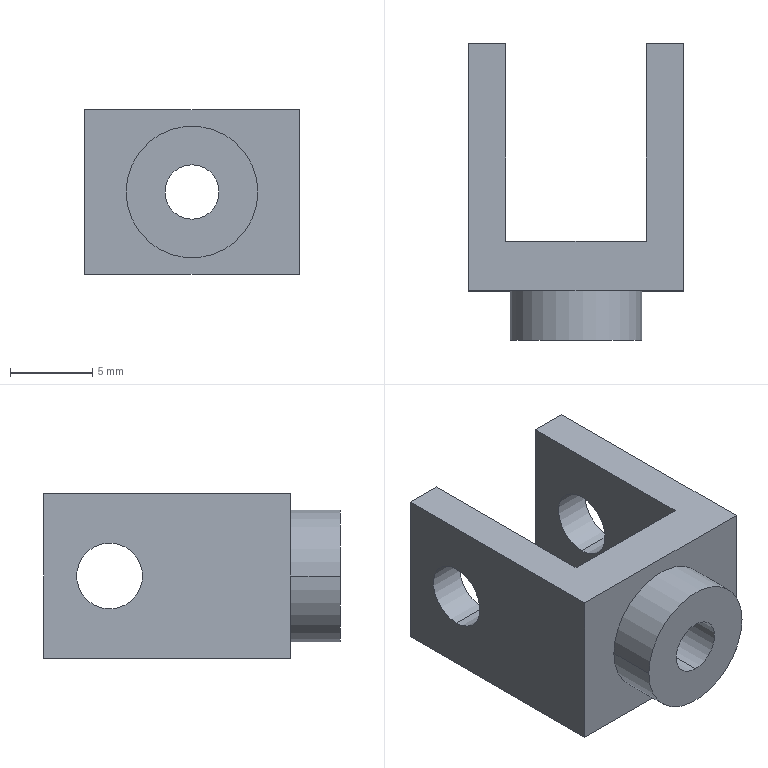Part | SolidWorks | features ICE 3, 3DProfileFeature 1, Extrusion 1, HoleWzd 1 | 1 solid | 19 faces | box 13 x 18 x 10 mm | volume 972.93 mm3 | plane 11 | cylinder 8 | commonest cylinder face diameters 4 x4 3.3 x2 8 x2
STEP:
#1=CARTESIAN_POINT('',(0.,-4.5,1.65));
#2=VERTEX_POINT('',#1);
#3=CARTESIAN_POINT('',(0.,-4.5,-1.65));
#4=VERTEX_POINT('',#3);
#5=CARTESIAN_POINT('',(0.,-4.5,0.));
#6=DIRECTION('',(0.,-1.,0.));
#7=DIRECTION('',(1.,0.,0.));
#8=AXIS2_PLACEMENT_3D('',#5,#6,#7);
#9=CIRCLE('',#8,1.65);
#10=EDGE_CURVE('',#2,#4,#9,.T.);
#11=ORIENTED_EDGE('',*,*,#10,.F.);
#12=CARTESIAN_POINT('',(0.,-10.5,1.65));
#13=VERTEX_POINT('',#12);
#14=CARTESIAN_POINT('',(0.,-10.5,1.65));
#15=DIRECTION('',(0.,-1.,0.));
#16=VECTOR('',#15,1000.);
#17=LINE('',#14,#16);
#18=EDGE_CURVE('',#2,#13,#17,.T.);
#19=ORIENTED_EDGE('',*,*,#18,.T.);
#20=CARTESIAN_POINT('',(0.,-10.5,-1.65));
#21=VERTEX_POINT('',#20);
#22=CARTESIAN_POINT('',(0.,-10.5,0.));
#23=DIRECTION('',(0.,-1.,0.));
#24=DIRECTION('',(0.,0.,-1.));
#25=AXIS2_PLACEMENT_3D('',#22,#23,#24);
#26=CIRCLE('',#25,1.65);
#27=EDGE_CURVE('',#13,#21,#26,.T.);
#28=ORIENTED_EDGE('',*,*,#27,.T.);
#29=CARTESIAN_POINT('',(0.,-10.5,-1.65));
#30=DIRECTION('',(0.,-1.,0.));
#31=VECTOR('',#30,1000.);
#32=LINE('',#29,#31);
#33=EDGE_CURVE('',#4,#21,#32,.T.);
#34=ORIENTED_EDGE('',*,*,#33,.F.);
#35=EDGE_LOOP('',(#11,#19,#28,#34));
#36=FACE_OUTER_BOUND('',#35,.T.);
#37=CARTESIAN_POINT('',(0.,-10.5,0.));
#38=DIRECTION('',(0.,-1.,0.));
#39=DIRECTION('',(0.,0.,-1.));
#40=AXIS2_PLACEMENT_3D('',#37,#38,#39);
#41=CYLINDRICAL_SURFACE('',#40,1.65);
#42=ADVANCED_FACE('',(#36),#41,.F.);
#43=CARTESIAN_POINT('',(4.,-10.5,0.));
#44=VERTEX_POINT('',#43);
#45=CARTESIAN_POINT('',(-4.,-10.5,0.));
#46=VERTEX_POINT('',#45);
#47=CARTESIAN_POINT('',(0.,-10.5,0.));
#48=DIRECTION('',(0.,-1.,0.));
#49=DIRECTION('',(1.,0.,0.));
#50=AXIS2_PLACEMENT_3D('',#47,#48,#49);
#51=CIRCLE('',#50,4.);
#52=EDGE_CURVE('',#44,#46,#51,.T.);
#53=ORIENTED_EDGE('',*,*,#52,.F.);
#54=CARTESIAN_POINT('',(4.,-7.5,0.));
#55=VERTEX_POINT('',#54);
#56=CARTESIAN_POINT('',(4.,-10.5,0.));
#57=DIRECTION('',(0.,1.,0.));
#58=VECTOR('',#57,1000.);
#59=LINE('',#56,#58);
#60=EDGE_CURVE('',#44,#55,#59,.T.);
#61=ORIENTED_EDGE('',*,*,#60,.T.);
#62=CARTESIAN_POINT('',(-4.,-7.5,0.));
#63=VERTEX_POINT('',#62);
#64=CARTESIAN_POINT('',(0.,-7.5,0.));
#65=DIRECTION('',(0.,-1.,0.));
#66=DIRECTION('',(1.,0.,0.));
#67=AXIS2_PLACEMENT_3D('',#64,#65,#66);
#68=CIRCLE('',#67,4.);
#69=EDGE_CURVE('',#55,#63,#68,.T.);
#70=ORIENTED_EDGE('',*,*,#69,.T.);
#71=CARTESIAN_POINT('',(-4.,-10.5,0.));
#72=DIRECTION('',(0.,1.,0.));
#73=VECTOR('',#72,1000.);
#74=LINE('',#71,#73);
#75=EDGE_CURVE('',#46,#63,#74,.T.);
#76=ORIENTED_EDGE('',*,*,#75,.F.);
#77=EDGE_LOOP('',(#53,#61,#70,#76));
#78=FACE_OUTER_BOUND('',#77,.T.);
#79=CARTESIAN_POINT('',(0.,-10.5,0.));
#80=DIRECTION('',(0.,1.,0.));
#81=DIRECTION('',(-1.,0.,0.));
#82=AXIS2_PLACEMENT_3D('',#79,#80,#81);
#83=CYLINDRICAL_SURFACE('',#82,4.);
#84=ADVANCED_FACE('',(#78),#83,.T.);
#85=CARTESIAN_POINT('',(-6.5,3.5,2.));
#86=VERTEX_POINT('',#85);
#87=CARTESIAN_POINT('',(-6.5,3.5,-2.));
#88=VERTEX_POINT('',#87);
#89=CARTESIAN_POINT('',(-6.5,3.5,0.));
#90=DIRECTION('',(1.,0.,0.));
#91=DIRECTION('',(0.,0.,-1.));
#92=AXIS2_PLACEMENT_3D('',#89,#90,#91);
#93=CIRCLE('',#92,2.);
#94=EDGE_CURVE('',#86,#88,#93,.T.);
#95=ORIENTED_EDGE('',*,*,#94,.F.);
#96=CARTESIAN_POINT('',(-4.25,3.5,2.));
#97=VERTEX_POINT('',#96);
#98=CARTESIAN_POINT('',(-18.5,3.5,2.));
#99=DIRECTION('',(1.,0.,0.));
#100=VECTOR('',#99,1000.);
#101=LINE('',#98,#100);
#102=EDGE_CURVE('',#86,#97,#101,.T.);
#103=ORIENTED_EDGE('',*,*,#102,.T.);
#104=CARTESIAN_POINT('',(-4.25,3.5,-2.));
#105=VERTEX_POINT('',#104);
#106=CARTESIAN_POINT('',(-4.25,3.5,0.));
#107=DIRECTION('',(-1.,0.,0.));
#108=DIRECTION('',(0.,0.,1.));
#109=AXIS2_PLACEMENT_3D('',#106,#107,#108);
#110=CIRCLE('',#109,2.);
#111=EDGE_CURVE('',#105,#97,#110,.T.);
#112=ORIENTED_EDGE('',*,*,#111,.F.);
#113=CARTESIAN_POINT('',(-18.5,3.5,-2.));
#114=DIRECTION('',(1.,0.,0.));
#115=VECTOR('',#114,1000.);
#116=LINE('',#113,#115);
#117=EDGE_CURVE('',#88,#105,#116,.T.);
#118=ORIENTED_EDGE('',*,*,#117,.F.);
#119=EDGE_LOOP('',(#95,#103,#112,#118));
#120=FACE_OUTER_BOUND('',#119,.T.);
#121=CARTESIAN_POINT('',(-18.5,3.5,0.));
#122=DIRECTION('',(1.,0.,0.));
#123=DIRECTION('',(0.,0.,-1.));
#124=AXIS2_PLACEMENT_3D('',#121,#122,#123);
#125=CYLINDRICAL_SURFACE('',#124,2.);
#126=ADVANCED_FACE('',(#120),#125,.F.);
#127=CARTESIAN_POINT('',(4.25,3.5,2.));
#128=VERTEX_POINT('',#127);
#129=CARTESIAN_POINT('',(4.25,3.5,-2.));
#130=VERTEX_POINT('',#129);
#131=CARTESIAN_POINT('',(4.25,3.5,0.));
#132=DIRECTION('',(1.,0.,0.));
#133=DIRECTION('',(0.,1.,0.));
#134=AXIS2_PLACEMENT_3D('',#131,#132,#133);
#135=CIRCLE('',#134,2.);
#136=EDGE_CURVE('',#128,#130,#135,.T.);
#137=ORIENTED_EDGE('',*,*,#136,.F.);
#138=CARTESIAN_POINT('',(6.5,3.5,2.));
#139=VERTEX_POINT('',#138);
#140=CARTESIAN_POINT('',(-18.5,3.5,2.));
#141=DIRECTION('',(1.,0.,0.));
#142=VECTOR('',#141,1000.);
#143=LINE('',#140,#142);
#144=EDGE_CURVE('',#128,#139,#143,.T.);
#145=ORIENTED_EDGE('',*,*,#144,.T.);
#146=CARTESIAN_POINT('',(6.5,3.5,-2.));
#147=VERTEX_POINT('',#146);
#148=CARTESIAN_POINT('',(6.5,3.5,0.));
#149=DIRECTION('',(1.,0.,0.));
#150=DIRECTION('',(0.,0.,-1.));
#151=AXIS2_PLACEMENT_3D('',#148,#149,#150);
#152=CIRCLE('',#151,2.);
#153=EDGE_CURVE('',#139,#147,#152,.T.);
#154=ORIENTED_EDGE('',*,*,#153,.T.);
#155=CARTESIAN_POINT('',(-18.5,3.5,-2.));
#156=DIRECTION('',(1.,0.,0.));
#157=VECTOR('',#156,1000.);
#158=LINE('',#155,#157);
#159=EDGE_CURVE('',#130,#147,#158,.T.);
#160=ORIENTED_EDGE('',*,*,#159,.F.);
#161=EDGE_LOOP('',(#137,#145,#154,#160));
#162=FACE_OUTER_BOUND('',#161,.T.);
#163=CARTESIAN_POINT('',(-18.5,3.5,0.));
#164=DIRECTION('',(1.,0.,0.));
#165=DIRECTION('',(0.,0.,-1.));
#166=AXIS2_PLACEMENT_3D('',#163,#164,#165);
#167=CYLINDRICAL_SURFACE('',#166,2.);
#168=ADVANCED_FACE('',(#162),#167,.F.);
#169=CARTESIAN_POINT('',(-4.25,7.5,5.));
#170=VERTEX_POINT('',#169);
#171=CARTESIAN_POINT('',(-6.5,7.5,5.));
#172=VERTEX_POINT('',#171);
#173=CARTESIAN_POINT('',(6.5,7.5,5.));
#174=DIRECTION('',(-1.,0.,0.));
#175=VECTOR('',#174,1000.);
#176=LINE('',#173,#175);
#177=EDGE_CURVE('',#170,#172,#176,.T.);
#178=ORIENTED_EDGE('',*,*,#177,.F.);
#179=CARTESIAN_POINT('',(-4.25,7.5,-5.));
#180=VERTEX_POINT('',#179);
#181=CARTESIAN_POINT('',(-4.25,7.5,5.));
#182=DIRECTION('',(0.,0.,-1.));
#183=VECTOR('',#182,1000.);
#184=LINE('',#181,#183);
#185=EDGE_CURVE('',#170,#180,#184,.T.);
#186=ORIENTED_EDGE('',*,*,#185,.T.);
#187=CARTESIAN_POINT('',(-6.5,7.5,-5.));
#188=VERTEX_POINT('',#187);
#189=CARTESIAN_POINT('',(6.5,7.5,-5.));
#190=DIRECTION('',(-1.,0.,0.));
#191=VECTOR('',#190,1000.);
#192=LINE('',#189,#191);
#193=EDGE_CURVE('',#180,#188,#192,.T.);
#194=ORIENTED_EDGE('',*,*,#193,.T.);
#195=CARTESIAN_POINT('',(-6.5,7.5,5.));
#196=DIRECTION('',(0.,0.,-1.));
#197=VECTOR('',#196,1000.);
#198=LINE('',#195,#197);
#199=EDGE_CURVE('',#172,#188,#198,.T.);
#200=ORIENTED_EDGE('',*,*,#199,.F.);
#201=EDGE_LOOP('',(#178,#186,#194,#200));
#202=FACE_OUTER_BOUND('',#201,.T.);
#203=CARTESIAN_POINT('',(6.5,7.5,5.));
#204=DIRECTION('',(0.,-1.,0.));
#205=DIRECTION('',(1.,0.,0.));
#206=AXIS2_PLACEMENT_3D('',#203,#204,#205);
#207=PLANE('',#206);
#208=ADVANCED_FACE('',(#202),#207,.F.);
#209=CARTESIAN_POINT('',(-6.5,3.5,0.));
#210=DIRECTION('',(1.,0.,0.));
#211=DIRECTION('',(0.,0.,-1.));
#212=AXIS2_PLACEMENT_3D('',#209,#210,#211);
#213=CIRCLE('',#212,2.);
#214=EDGE_CURVE('',#88,#86,#213,.T.);
#215=ORIENTED_EDGE('',*,*,#214,.T.);
#216=ORIENTED_EDGE('',*,*,#94,.T.);
#217=EDGE_LOOP('',(#215,#216));
#218=FACE_BOUND('',#217,.T.);
#219=CARTESIAN_POINT('',(-6.5,-7.5,-5.));
#220=VERTEX_POINT('',#219);
#221=CARTESIAN_POINT('',(-6.5,-7.5,-5.));
#222=DIRECTION('',(0.,-1.,0.));
#223=VECTOR('',#222,1000.);
#224=LINE('',#221,#223);
#225=EDGE_CURVE('',#188,#220,#224,.T.);
#226=ORIENTED_EDGE('',*,*,#225,.T.);
#227=CARTESIAN_POINT('',(-6.5,-7.5,5.));
#228=VERTEX_POINT('',#227);
#229=CARTESIAN_POINT('',(-6.5,-7.5,5.));
#230=DIRECTION('',(0.,0.,-1.));
#231=VECTOR('',#230,1000.);
#232=LINE('',#229,#231);
#233=EDGE_CURVE('',#228,#220,#232,.T.);
#234=ORIENTED_EDGE('',*,*,#233,.F.);
#235=CARTESIAN_POINT('',(-6.5,-7.5,5.));
#236=DIRECTION('',(0.,-1.,0.));
#237=VECTOR('',#236,1000.);
#238=LINE('',#235,#237);
#239=EDGE_CURVE('',#172,#228,#238,.T.);
#240=ORIENTED_EDGE('',*,*,#239,.F.);
#241=ORIENTED_EDGE('',*,*,#199,.T.);
#242=EDGE_LOOP('',(#226,#234,#240,#241));
#243=FACE_OUTER_BOUND('',#242,.T.);
#244=CARTESIAN_POINT('',(-6.5,-7.5,5.));
#245=DIRECTION('',(1.,0.,0.));
#246=DIRECTION('',(0.,0.,-1.));
#247=AXIS2_PLACEMENT_3D('',#244,#245,#246);
#248=PLANE('',#247);
#249=ADVANCED_FACE('',(#218,#243),#248,.F.);
#250=CARTESIAN_POINT('',(0.,-7.5,0.));
#251=DIRECTION('',(0.,-1.,0.));
#252=DIRECTION('',(1.,0.,0.));
#253=AXIS2_PLACEMENT_3D('',#250,#251,#252);
#254=CIRCLE('',#253,4.);
#255=EDGE_CURVE('',#63,#55,#254,.T.);
#256=ORIENTED_EDGE('',*,*,#255,.F.);
#257=ORIENTED_EDGE('',*,*,#69,.F.);
#258=EDGE_LOOP('',(#256,#257));
#259=FACE_BOUND('',#258,.T.);
#260=CARTESIAN_POINT('',(6.5,-7.5,-5.));
#261=VERTEX_POINT('',#260);
#262=CARTESIAN_POINT('',(6.5,-7.5,-5.));
#263=DIRECTION('',(1.,0.,0.));
#264=VECTOR('',#263,1000.);
#265=LINE('',#262,#264);
#266=EDGE_CURVE('',#220,#261,#265,.T.);
#267=ORIENTED_EDGE('',*,*,#266,.T.);
#268=CARTESIAN_POINT('',(6.5,-7.5,5.));
#269=VERTEX_POINT('',#268);
#270=CARTESIAN_POINT('',(6.5,-7.5,5.));
#271=DIRECTION('',(0.,0.,-1.));
#272=VECTOR('',#271,1000.);
#273=LINE('',#270,#272);
#274=EDGE_CURVE('',#269,#261,#273,.T.);
#275=ORIENTED_EDGE('',*,*,#274,.F.);
#276=CARTESIAN_POINT('',(6.5,-7.5,5.));
#277=DIRECTION('',(1.,0.,0.));
#278=VECTOR('',#277,1000.);
#279=LINE('',#276,#278);
#280=EDGE_CURVE('',#228,#269,#279,.T.);
#281=ORIENTED_EDGE('',*,*,#280,.F.);
#282=ORIENTED_EDGE('',*,*,#233,.T.);
#283=EDGE_LOOP('',(#267,#275,#281,#282));
#284=FACE_OUTER_BOUND('',#283,.T.);
#285=CARTESIAN_POINT('',(6.5,-7.5,5.));
#286=DIRECTION('',(0.,1.,0.));
#287=DIRECTION('',(-1.,0.,0.));
#288=AXIS2_PLACEMENT_3D('',#285,#286,#287);
#289=PLANE('',#288);
#290=ADVANCED_FACE('',(#259,#284),#289,.F.);
#291=CARTESIAN_POINT('',(6.5,3.5,0.));
#292=DIRECTION('',(1.,0.,0.));
#293=DIRECTION('',(0.,0.,-1.));
#294=AXIS2_PLACEMENT_3D('',#291,#292,#293);
#295=CIRCLE('',#294,2.);
#296=EDGE_CURVE('',#147,#139,#295,.T.);
#297=ORIENTED_EDGE('',*,*,#296,.F.);
#298=ORIENTED_EDGE('',*,*,#153,.F.);
#299=EDGE_LOOP('',(#297,#298));
#300=FACE_BOUND('',#299,.T.);
#301=CARTESIAN_POINT('',(6.5,7.5,-5.));
#302=VERTEX_POINT('',#301);
#303=CARTESIAN_POINT('',(6.5,-7.5,-5.));
#304=DIRECTION('',(0.,1.,0.));
#305=VECTOR('',#304,1000.);
#306=LINE('',#303,#305);
#307=EDGE_CURVE('',#261,#302,#306,.T.);
#308=ORIENTED_EDGE('',*,*,#307,.T.);
#309=CARTESIAN_POINT('',(6.5,7.5,5.));
#310=VERTEX_POINT('',#309);
#311=CARTESIAN_POINT('',(6.5,7.5,5.));
#312=DIRECTION('',(0.,0.,-1.));
#313=VECTOR('',#312,1000.);
#314=LINE('',#311,#313);
#315=EDGE_CURVE('',#310,#302,#314,.T.);
#316=ORIENTED_EDGE('',*,*,#315,.F.);
#317=CARTESIAN_POINT('',(6.5,-7.5,5.));
#318=DIRECTION('',(0.,1.,0.));
#319=VECTOR('',#318,1000.);
#320=LINE('',#317,#319);
#321=EDGE_CURVE('',#269,#310,#320,.T.);
#322=ORIENTED_EDGE('',*,*,#321,.F.);
#323=ORIENTED_EDGE('',*,*,#274,.T.);
#324=EDGE_LOOP('',(#308,#316,#322,#323));
#325=FACE_OUTER_BOUND('',#324,.T.);
#326=CARTESIAN_POINT('',(6.5,-7.5,5.));
#327=DIRECTION('',(-1.,0.,0.));
#328=DIRECTION('',(0.,0.,1.));
#329=AXIS2_PLACEMENT_3D('',#326,#327,#328);
#330=PLANE('',#329);
#331=ADVANCED_FACE('',(#300,#325),#330,.F.);
#332=CARTESIAN_POINT('',(4.25,7.5,-5.));
#333=VERTEX_POINT('',#332);
#334=CARTESIAN_POINT('',(6.5,7.5,-5.));
#335=DIRECTION('',(-1.,0.,0.));
#336=VECTOR('',#335,1000.);
#337=LINE('',#334,#336);
#338=EDGE_CURVE('',#302,#333,#337,.T.);
#339=ORIENTED_EDGE('',*,*,#338,.T.);
#340=CARTESIAN_POINT('',(4.25,7.5,5.));
#341=VERTEX_POINT('',#340);
#342=CARTESIAN_POINT('',(4.25,7.5,5.));
#343=DIRECTION('',(0.,0.,1.));
#344=VECTOR('',#343,1000.);
#345=LINE('',#342,#344);
#346=EDGE_CURVE('',#333,#341,#345,.T.);
#347=ORIENTED_EDGE('',*,*,#346,.T.);
#348=CARTESIAN_POINT('',(6.5,7.5,5.));
#349=DIRECTION('',(-1.,0.,0.));
#350=VECTOR('',#349,1000.);
#351=LINE('',#348,#350);
#352=EDGE_CURVE('',#310,#341,#351,.T.);
#353=ORIENTED_EDGE('',*,*,#352,.F.);
#354=ORIENTED_EDGE('',*,*,#315,.T.);
#355=EDGE_LOOP('',(#339,#347,#353,#354));
#356=FACE_OUTER_BOUND('',#355,.T.);
#357=CARTESIAN_POINT('',(6.5,7.5,5.));
#358=DIRECTION('',(0.,-1.,0.));
#359=DIRECTION('',(1.,0.,0.));
#360=AXIS2_PLACEMENT_3D('',#357,#358,#359);
#361=PLANE('',#360);
#362=ADVANCED_FACE('',(#356),#361,.F.);
#363=CARTESIAN_POINT('',(-4.25,-4.5,5.));
#364=VERTEX_POINT('',#363);
#365=CARTESIAN_POINT('',(-4.25,19.5,5.));
#366=DIRECTION('',(0.,-1.,0.));
#367=VECTOR('',#366,1000.);
#368=LINE('',#365,#367);
#369=EDGE_CURVE('',#170,#364,#368,.T.);
#370=ORIENTED_EDGE('',*,*,#369,.F.);
#371=ORIENTED_EDGE('',*,*,#177,.T.);
#372=ORIENTED_EDGE('',*,*,#239,.T.);
#373=ORIENTED_EDGE('',*,*,#280,.T.);
#374=ORIENTED_EDGE('',*,*,#321,.T.);
#375=ORIENTED_EDGE('',*,*,#352,.T.);
#376=CARTESIAN_POINT('',(4.25,-4.5,5.));
#377=VERTEX_POINT('',#376);
#378=CARTESIAN_POINT('',(4.25,19.5,5.));
#379=DIRECTION('',(0.,1.,0.));
#380=VECTOR('',#379,1000.);
#381=LINE('',#378,#380);
#382=EDGE_CURVE('',#377,#341,#381,.T.);
#383=ORIENTED_EDGE('',*,*,#382,.F.);
#384=CARTESIAN_POINT('',(4.25,-4.5,5.));
#385=DIRECTION('',(1.,0.,0.));
#386=VECTOR('',#385,1000.);
#387=LINE('',#384,#386);
#388=EDGE_CURVE('',#364,#377,#387,.T.);
#389=ORIENTED_EDGE('',*,*,#388,.F.);
#390=EDGE_LOOP('',(#370,#371,#372,#373,#374,#375,#383,#389));
#391=FACE_OUTER_BOUND('',#390,.T.);
#392=CARTESIAN_POINT('',(0.,0.,5.));
#393=DIRECTION('',(0.,0.,1.));
#394=DIRECTION('',(1.,0.,0.));
#395=AXIS2_PLACEMENT_3D('',#392,#393,#394);
#396=PLANE('',#395);
#397=ADVANCED_FACE('',(#391),#396,.T.);
#398=ORIENTED_EDGE('',*,*,#193,.F.);
#399=CARTESIAN_POINT('',(-4.25,-4.5,-5.));
#400=VERTEX_POINT('',#399);
#401=CARTESIAN_POINT('',(-4.25,0.,-5.));
#402=DIRECTION('',(0.,-1.,0.));
#403=VECTOR('',#402,1000.);
#404=LINE('',#401,#403);
#405=EDGE_CURVE('',#180,#400,#404,.T.);
#406=ORIENTED_EDGE('',*,*,#405,.T.);
#407=CARTESIAN_POINT('',(4.25,-4.5,-5.));
#408=VERTEX_POINT('',#407);
#409=CARTESIAN_POINT('',(4.25,-4.5,-5.));
#410=DIRECTION('',(1.,0.,0.));
#411=VECTOR('',#410,1000.);
#412=LINE('',#409,#411);
#413=EDGE_CURVE('',#400,#408,#412,.T.);
#414=ORIENTED_EDGE('',*,*,#413,.T.);
#415=CARTESIAN_POINT('',(4.25,19.5,-5.));
#416=DIRECTION('',(0.,1.,0.));
#417=VECTOR('',#416,1000.);
#418=LINE('',#415,#417);
#419=EDGE_CURVE('',#408,#333,#418,.T.);
#420=ORIENTED_EDGE('',*,*,#419,.T.);
#421=ORIENTED_EDGE('',*,*,#338,.F.);
#422=ORIENTED_EDGE('',*,*,#307,.F.);
#423=ORIENTED_EDGE('',*,*,#266,.F.);
#424=ORIENTED_EDGE('',*,*,#225,.F.);
#425=EDGE_LOOP('',(#398,#406,#414,#420,#421,#422,#423,#424));
#426=FACE_OUTER_BOUND('',#425,.T.);
#427=CARTESIAN_POINT('',(0.,0.,-5.));
#428=DIRECTION('',(0.,0.,1.));
#429=DIRECTION('',(1.,0.,0.));
#430=AXIS2_PLACEMENT_3D('',#427,#428,#429);
#431=PLANE('',#430);
#432=ADVANCED_FACE('',(#426),#431,.F.);
#433=ORIENTED_EDGE('',*,*,#111,.T.);
#434=CARTESIAN_POINT('',(-4.25,3.5,0.));
#435=DIRECTION('',(-1.,0.,0.));
#436=DIRECTION('',(0.,0.,1.));
#437=AXIS2_PLACEMENT_3D('',#434,#435,#436);
#438=CIRCLE('',#437,2.);
#439=EDGE_CURVE('',#97,#105,#438,.T.);
#440=ORIENTED_EDGE('',*,*,#439,.T.);
#441=EDGE_LOOP('',(#433,#440));
#442=FACE_BOUND('',#441,.T.);
#443=ORIENTED_EDGE('',*,*,#369,.T.);
#444=CARTESIAN_POINT('',(-4.25,-4.5,-5.));
#445=DIRECTION('',(0.,0.,1.));
#446=VECTOR('',#445,1000.);
#447=LINE('',#444,#446);
#448=EDGE_CURVE('',#400,#364,#447,.T.);
#449=ORIENTED_EDGE('',*,*,#448,.F.);
#450=ORIENTED_EDGE('',*,*,#405,.F.);
#451=ORIENTED_EDGE('',*,*,#185,.F.);
#452=EDGE_LOOP('',(#443,#449,#450,#451));
#453=FACE_OUTER_BOUND('',#452,.T.);
#454=CARTESIAN_POINT('',(-4.25,19.5,-5.));
#455=DIRECTION('',(-1.,0.,0.));
#456=DIRECTION('',(0.,0.,1.));
#457=AXIS2_PLACEMENT_3D('',#454,#455,#456);
#458=PLANE('',#457);
#459=ADVANCED_FACE('',(#442,#453),#458,.F.);
#460=CARTESIAN_POINT('',(4.25,3.5,0.));
#461=DIRECTION('',(1.,0.,0.));
#462=DIRECTION('',(0.,1.,0.));
#463=AXIS2_PLACEMENT_3D('',#460,#461,#462);
#464=CIRCLE('',#463,2.);
#465=EDGE_CURVE('',#130,#128,#464,.T.);
#466=ORIENTED_EDGE('',*,*,#465,.T.);
#467=ORIENTED_EDGE('',*,*,#136,.T.);
#468=EDGE_LOOP('',(#466,#467));
#469=FACE_BOUND('',#468,.T.);
#470=ORIENTED_EDGE('',*,*,#419,.F.);
#471=CARTESIAN_POINT('',(4.25,-4.5,-5.));
#472=DIRECTION('',(0.,0.,1.));
#473=VECTOR('',#472,1000.);
#474=LINE('',#471,#473);
#475=EDGE_CURVE('',#408,#377,#474,.T.);
#476=ORIENTED_EDGE('',*,*,#475,.T.);
#477=ORIENTED_EDGE('',*,*,#382,.T.);
#478=ORIENTED_EDGE('',*,*,#346,.F.);
#479=EDGE_LOOP('',(#470,#476,#477,#478));
#480=FACE_OUTER_BOUND('',#479,.T.);
#481=CARTESIAN_POINT('',(4.25,19.5,-5.));
#482=DIRECTION('',(1.,0.,0.));
#483=DIRECTION('',(0.,1.,0.));
#484=AXIS2_PLACEMENT_3D('',#481,#482,#483);
#485=PLANE('',#484);
#486=ADVANCED_FACE('',(#469,#480),#485,.F.);
#487=CARTESIAN_POINT('',(0.,-4.5,0.));
#488=DIRECTION('',(0.,-1.,0.));
#489=DIRECTION('',(1.,0.,0.));
#490=AXIS2_PLACEMENT_3D('',#487,#488,#489);
#491=CIRCLE('',#490,1.65);
#492=EDGE_CURVE('',#4,#2,#491,.T.);
#493=ORIENTED_EDGE('',*,*,#492,.T.);
#494=ORIENTED_EDGE('',*,*,#10,.T.);
#495=EDGE_LOOP('',(#493,#494));
#496=FACE_BOUND('',#495,.T.);
#497=ORIENTED_EDGE('',*,*,#388,.T.);
#498=ORIENTED_EDGE('',*,*,#475,.F.);
#499=ORIENTED_EDGE('',*,*,#413,.F.);
#500=ORIENTED_EDGE('',*,*,#448,.T.);
#501=EDGE_LOOP('',(#497,#498,#499,#500));
#502=FACE_OUTER_BOUND('',#501,.T.);
#503=CARTESIAN_POINT('',(4.25,-4.5,-5.));
#504=DIRECTION('',(0.,-1.,0.));
#505=DIRECTION('',(1.,0.,0.));
#506=AXIS2_PLACEMENT_3D('',#503,#504,#505);
#507=PLANE('',#506);
#508=ADVANCED_FACE('',(#496,#502),#507,.F.);
#509=ORIENTED_EDGE('',*,*,#144,.F.);
#510=ORIENTED_EDGE('',*,*,#465,.F.);
#511=ORIENTED_EDGE('',*,*,#159,.T.);
#512=ORIENTED_EDGE('',*,*,#296,.T.);
#513=EDGE_LOOP('',(#509,#510,#511,#512));
#514=FACE_OUTER_BOUND('',#513,.T.);
#515=CARTESIAN_POINT('',(-18.5,3.5,0.));
#516=DIRECTION('',(1.,0.,0.));
#517=DIRECTION('',(0.,0.,-1.));
#518=AXIS2_PLACEMENT_3D('',#515,#516,#517);
#519=CYLINDRICAL_SURFACE('',#518,2.);
#520=ADVANCED_FACE('',(#514),#519,.F.);
#521=ORIENTED_EDGE('',*,*,#102,.F.);
#522=ORIENTED_EDGE('',*,*,#214,.F.);
#523=ORIENTED_EDGE('',*,*,#117,.T.);
#524=ORIENTED_EDGE('',*,*,#439,.F.);
#525=EDGE_LOOP('',(#521,#522,#523,#524));
#526=FACE_OUTER_BOUND('',#525,.T.);
#527=CARTESIAN_POINT('',(-18.5,3.5,0.));
#528=DIRECTION('',(1.,0.,0.));
#529=DIRECTION('',(0.,0.,-1.));
#530=AXIS2_PLACEMENT_3D('',#527,#528,#529);
#531=CYLINDRICAL_SURFACE('',#530,2.);
#532=ADVANCED_FACE('',(#526),#531,.F.);
#533=ORIENTED_EDGE('',*,*,#60,.F.);
#534=CARTESIAN_POINT('',(0.,-10.5,0.));
#535=DIRECTION('',(0.,-1.,0.));
#536=DIRECTION('',(1.,0.,0.));
#537=AXIS2_PLACEMENT_3D('',#534,#535,#536);
#538=CIRCLE('',#537,4.);
#539=EDGE_CURVE('',#46,#44,#538,.T.);
#540=ORIENTED_EDGE('',*,*,#539,.F.);
#541=ORIENTED_EDGE('',*,*,#75,.T.);
#542=ORIENTED_EDGE('',*,*,#255,.T.);
#543=EDGE_LOOP('',(#533,#540,#541,#542));
#544=FACE_OUTER_BOUND('',#543,.T.);
#545=CARTESIAN_POINT('',(0.,-10.5,0.));
#546=DIRECTION('',(0.,1.,0.));
#547=DIRECTION('',(-1.,0.,0.));
#548=AXIS2_PLACEMENT_3D('',#545,#546,#547);
#549=CYLINDRICAL_SURFACE('',#548,4.);
#550=ADVANCED_FACE('',(#544),#549,.T.);
#551=CARTESIAN_POINT('',(0.,-10.5,0.));
#552=DIRECTION('',(0.,-1.,0.));
#553=DIRECTION('',(0.,0.,-1.));
#554=AXIS2_PLACEMENT_3D('',#551,#552,#553);
#555=CIRCLE('',#554,1.65);
#556=EDGE_CURVE('',#21,#13,#555,.T.);
#557=ORIENTED_EDGE('',*,*,#556,.F.);
#558=ORIENTED_EDGE('',*,*,#27,.F.);
#559=EDGE_LOOP('',(#557,#558));
#560=FACE_BOUND('',#559,.T.);
#561=ORIENTED_EDGE('',*,*,#539,.T.);
#562=ORIENTED_EDGE('',*,*,#52,.T.);
#563=EDGE_LOOP('',(#561,#562));
#564=FACE_OUTER_BOUND('',#563,.T.);
#565=CARTESIAN_POINT('',(0.,-10.5,0.));
#566=DIRECTION('',(0.,-1.,0.));
#567=DIRECTION('',(1.,0.,0.));
#568=AXIS2_PLACEMENT_3D('',#565,#566,#567);
#569=PLANE('',#568);
#570=ADVANCED_FACE('',(#560,#564),#569,.T.);
#571=ORIENTED_EDGE('',*,*,#18,.F.);
#572=ORIENTED_EDGE('',*,*,#492,.F.);
#573=ORIENTED_EDGE('',*,*,#33,.T.);
#574=ORIENTED_EDGE('',*,*,#556,.T.);
#575=EDGE_LOOP('',(#571,#572,#573,#574));
#576=FACE_OUTER_BOUND('',#575,.T.);
#577=CARTESIAN_POINT('',(0.,-10.5,0.));
#578=DIRECTION('',(0.,-1.,0.));
#579=DIRECTION('',(0.,0.,-1.));
#580=AXIS2_PLACEMENT_3D('',#577,#578,#579);
#581=CYLINDRICAL_SURFACE('',#580,1.65);
#582=ADVANCED_FACE('',(#576),#581,.F.);
#583=CLOSED_SHELL('',(#42,#84,#126,#168,#208,#249,#290,#331,#362,#397,#432,#459,#486,#508,#520,#532,#550,#570,#582));
#584=MANIFOLD_SOLID_BREP('',#583);
#585=CARTESIAN_POINT('',(0.,0.,0.));
#586=DIRECTION('',(0.,0.,1.));
#587=DIRECTION('',(1.,0.,0.));
#588=AXIS2_PLACEMENT_3D('',#585,#586,#587);
#589=(LENGTH_UNIT()NAMED_UNIT(*)SI_UNIT(.MILLI.,.METRE.));
#590=UNCERTAINTY_MEASURE_WITH_UNIT(LENGTH_MEASURE(0.00001),#589,'','');
#591=(NAMED_UNIT(*)PLANE_ANGLE_UNIT()SI_UNIT($,.RADIAN.));
#592=(NAMED_UNIT(*)SI_UNIT($,.STERADIAN.)SOLID_ANGLE_UNIT());
#593=(GEOMETRIC_REPRESENTATION_CONTEXT(3)GLOBAL_UNCERTAINTY_ASSIGNED_CONTEXT((#590))GLOBAL_UNIT_ASSIGNED_CONTEXT((#589,#591,#592))REPRESENTATION_CONTEXT('',''));
#594=ADVANCED_BREP_SHAPE_REPRESENTATION('',(#584,#588),#593);